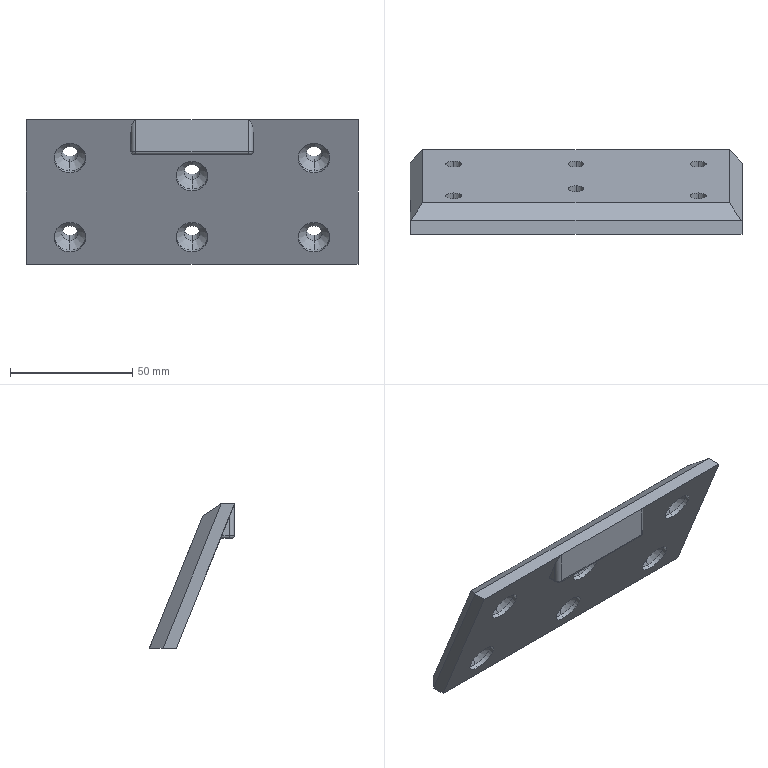Part | Creo | 1 solid | 56 faces | box 136 x 34.785 x 59 mm | volume 82719 mm3 | cylinder 29 | plane 13 | cone 12 | spline 2 | commonest cylinder face diameters 6.6 x12 13 x12 2 x3 4 x2